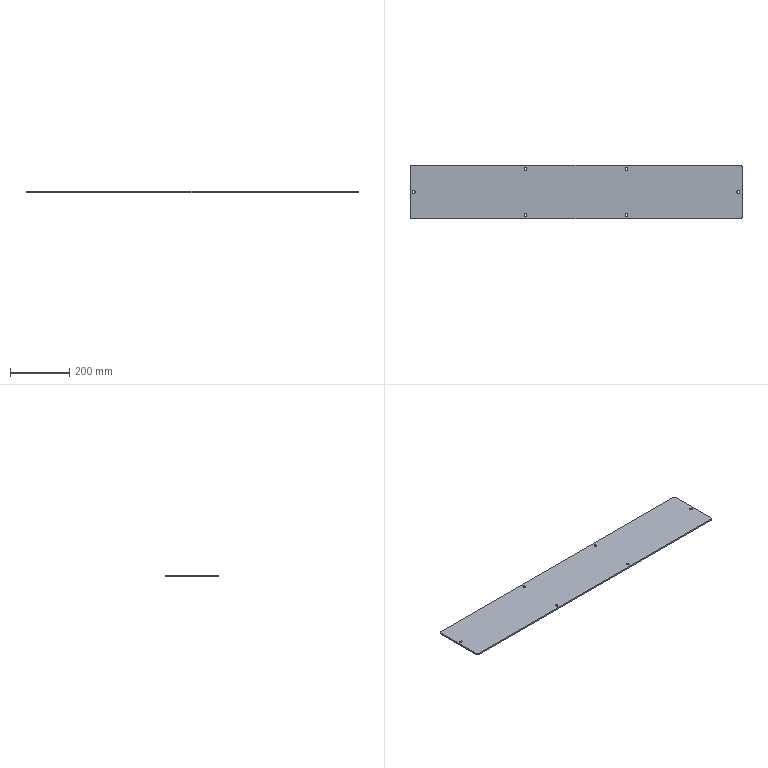Part | STEP file | 1 solid | 36 faces | box 1119 x 179 x 5 mm | volume 999682 mm3 | cylinder 18 | plane 18 | commonest cylinder face diameters 7 x14 6 x4